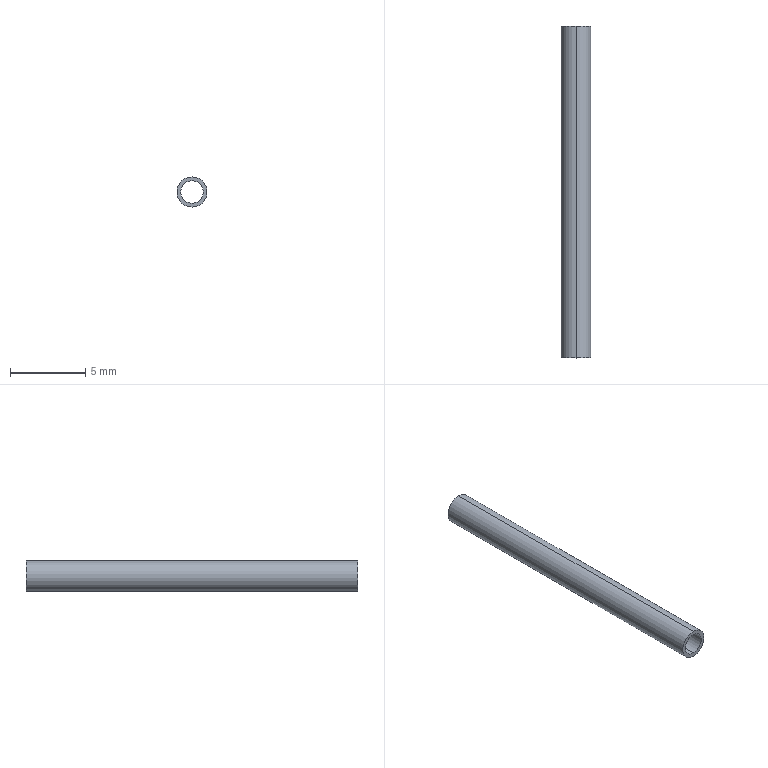Part | SolidWorks | features Revolution 1 | 1 solid | 6 faces | box 2 x 22 x 2 mm | volume 30.238 mm3 | cylinder 4 | plane 2 | commonest cylinder face diameters 1.5 x2 2 x2
STEP:
#1=CARTESIAN_POINT('',(0.,10.2,-1.));
#2=VERTEX_POINT('',#1);
#3=CARTESIAN_POINT('',(0.,10.2,1.));
#4=VERTEX_POINT('',#3);
#5=CARTESIAN_POINT('',(0.,10.2,0.));
#6=DIRECTION('',(0.,-1.,0.));
#7=DIRECTION('',(0.,0.,-1.));
#8=AXIS2_PLACEMENT_3D('',#5,#6,#7);
#9=CIRCLE('',#8,1.);
#10=EDGE_CURVE('',#2,#4,#9,.T.);
#11=ORIENTED_EDGE('',*,*,#10,.T.);
#12=CARTESIAN_POINT('',(0.,-11.8,1.));
#13=VERTEX_POINT('',#12);
#14=CARTESIAN_POINT('',(0.,-14.434,1.));
#15=DIRECTION('',(0.,-1.,0.));
#16=VECTOR('',#15,1000.);
#17=LINE('',#14,#16);
#18=EDGE_CURVE('',#4,#13,#17,.T.);
#19=ORIENTED_EDGE('',*,*,#18,.T.);
#20=CARTESIAN_POINT('',(0.,-11.8,-1.));
#21=VERTEX_POINT('',#20);
#22=CARTESIAN_POINT('',(0.,-11.8,0.));
#23=DIRECTION('',(0.,-1.,0.));
#24=DIRECTION('',(0.,0.,-1.));
#25=AXIS2_PLACEMENT_3D('',#22,#23,#24);
#26=CIRCLE('',#25,1.);
#27=EDGE_CURVE('',#21,#13,#26,.T.);
#28=ORIENTED_EDGE('',*,*,#27,.F.);
#29=CARTESIAN_POINT('',(0.,-14.434,-1.));
#30=DIRECTION('',(0.,-1.,0.));
#31=VECTOR('',#30,1000.);
#32=LINE('',#29,#31);
#33=EDGE_CURVE('',#2,#21,#32,.T.);
#34=ORIENTED_EDGE('',*,*,#33,.F.);
#35=EDGE_LOOP('',(#11,#19,#28,#34));
#36=FACE_OUTER_BOUND('',#35,.T.);
#37=CARTESIAN_POINT('',(0.,-14.434,0.));
#38=DIRECTION('',(0.,-1.,0.));
#39=DIRECTION('',(0.,0.,-1.));
#40=AXIS2_PLACEMENT_3D('',#37,#38,#39);
#41=CYLINDRICAL_SURFACE('',#40,1.);
#42=ADVANCED_FACE('',(#36),#41,.T.);
#43=CARTESIAN_POINT('',(0.,10.2,0.75));
#44=VERTEX_POINT('',#43);
#45=CARTESIAN_POINT('',(0.,10.2,-0.75));
#46=VERTEX_POINT('',#45);
#47=CARTESIAN_POINT('',(0.,10.2,0.));
#48=DIRECTION('',(0.,-1.,0.));
#49=DIRECTION('',(0.,0.,-1.));
#50=AXIS2_PLACEMENT_3D('',#47,#48,#49);
#51=CIRCLE('',#50,0.75);
#52=EDGE_CURVE('',#44,#46,#51,.T.);
#53=ORIENTED_EDGE('',*,*,#52,.F.);
#54=CARTESIAN_POINT('',(0.,-11.8,0.75));
#55=VERTEX_POINT('',#54);
#56=CARTESIAN_POINT('',(0.,-14.434,0.75));
#57=DIRECTION('',(0.,-1.,0.));
#58=VECTOR('',#57,1000.);
#59=LINE('',#56,#58);
#60=EDGE_CURVE('',#44,#55,#59,.T.);
#61=ORIENTED_EDGE('',*,*,#60,.T.);
#62=CARTESIAN_POINT('',(0.,-11.8,-0.75));
#63=VERTEX_POINT('',#62);
#64=CARTESIAN_POINT('',(0.,-11.8,0.));
#65=DIRECTION('',(0.,-1.,0.));
#66=DIRECTION('',(0.,0.,-1.));
#67=AXIS2_PLACEMENT_3D('',#64,#65,#66);
#68=CIRCLE('',#67,0.75);
#69=EDGE_CURVE('',#55,#63,#68,.T.);
#70=ORIENTED_EDGE('',*,*,#69,.T.);
#71=CARTESIAN_POINT('',(0.,-14.434,-0.75));
#72=DIRECTION('',(0.,-1.,0.));
#73=VECTOR('',#72,1000.);
#74=LINE('',#71,#73);
#75=EDGE_CURVE('',#46,#63,#74,.T.);
#76=ORIENTED_EDGE('',*,*,#75,.F.);
#77=EDGE_LOOP('',(#53,#61,#70,#76));
#78=FACE_OUTER_BOUND('',#77,.T.);
#79=CARTESIAN_POINT('',(0.,-14.434,0.));
#80=DIRECTION('',(0.,-1.,0.));
#81=DIRECTION('',(0.,0.,-1.));
#82=AXIS2_PLACEMENT_3D('',#79,#80,#81);
#83=CYLINDRICAL_SURFACE('',#82,0.75);
#84=ADVANCED_FACE('',(#78),#83,.F.);
#85=ORIENTED_EDGE('',*,*,#10,.F.);
#86=CARTESIAN_POINT('',(0.,10.2,0.));
#87=DIRECTION('',(0.,-1.,0.));
#88=DIRECTION('',(0.,0.,-1.));
#89=AXIS2_PLACEMENT_3D('',#86,#87,#88);
#90=CIRCLE('',#89,1.);
#91=EDGE_CURVE('',#4,#2,#90,.T.);
#92=ORIENTED_EDGE('',*,*,#91,.F.);
#93=EDGE_LOOP('',(#85,#92));
#94=FACE_OUTER_BOUND('',#93,.T.);
#95=CARTESIAN_POINT('',(0.,10.2,0.));
#96=DIRECTION('',(0.,-1.,0.));
#97=DIRECTION('',(0.,0.,-1.));
#98=AXIS2_PLACEMENT_3D('',#95,#96,#97);
#99=CIRCLE('',#98,0.75);
#100=EDGE_CURVE('',#46,#44,#99,.T.);
#101=ORIENTED_EDGE('',*,*,#100,.T.);
#102=ORIENTED_EDGE('',*,*,#52,.T.);
#103=EDGE_LOOP('',(#101,#102));
#104=FACE_BOUND('',#103,.T.);
#105=CARTESIAN_POINT('',(-1.,10.2,0.));
#106=DIRECTION('',(0.,-1.,0.));
#107=DIRECTION('',(0.,0.,-1.));
#108=AXIS2_PLACEMENT_3D('',#105,#106,#107);
#109=PLANE('',#108);
#110=ADVANCED_FACE('',(#94,#104),#109,.F.);
#111=ORIENTED_EDGE('',*,*,#60,.F.);
#112=ORIENTED_EDGE('',*,*,#100,.F.);
#113=ORIENTED_EDGE('',*,*,#75,.T.);
#114=CARTESIAN_POINT('',(0.,-11.8,0.));
#115=DIRECTION('',(0.,-1.,0.));
#116=DIRECTION('',(0.,0.,-1.));
#117=AXIS2_PLACEMENT_3D('',#114,#115,#116);
#118=CIRCLE('',#117,0.75);
#119=EDGE_CURVE('',#63,#55,#118,.T.);
#120=ORIENTED_EDGE('',*,*,#119,.T.);
#121=EDGE_LOOP('',(#111,#112,#113,#120));
#122=FACE_OUTER_BOUND('',#121,.T.);
#123=CARTESIAN_POINT('',(0.,-14.434,0.));
#124=DIRECTION('',(0.,-1.,0.));
#125=DIRECTION('',(0.,0.,-1.));
#126=AXIS2_PLACEMENT_3D('',#123,#124,#125);
#127=CYLINDRICAL_SURFACE('',#126,0.75);
#128=ADVANCED_FACE('',(#122),#127,.F.);
#129=ORIENTED_EDGE('',*,*,#119,.F.);
#130=ORIENTED_EDGE('',*,*,#69,.F.);
#131=EDGE_LOOP('',(#129,#130));
#132=FACE_BOUND('',#131,.T.);
#133=ORIENTED_EDGE('',*,*,#27,.T.);
#134=CARTESIAN_POINT('',(0.,-11.8,0.));
#135=DIRECTION('',(0.,-1.,0.));
#136=DIRECTION('',(0.,0.,-1.));
#137=AXIS2_PLACEMENT_3D('',#134,#135,#136);
#138=CIRCLE('',#137,1.);
#139=EDGE_CURVE('',#13,#21,#138,.T.);
#140=ORIENTED_EDGE('',*,*,#139,.T.);
#141=EDGE_LOOP('',(#133,#140));
#142=FACE_OUTER_BOUND('',#141,.T.);
#143=CARTESIAN_POINT('',(-1.,-11.8,0.));
#144=DIRECTION('',(0.,1.,0.));
#145=DIRECTION('',(0.,0.,1.));
#146=AXIS2_PLACEMENT_3D('',#143,#144,#145);
#147=PLANE('',#146);
#148=ADVANCED_FACE('',(#132,#142),#147,.F.);
#149=ORIENTED_EDGE('',*,*,#18,.F.);
#150=ORIENTED_EDGE('',*,*,#91,.T.);
#151=ORIENTED_EDGE('',*,*,#33,.T.);
#152=ORIENTED_EDGE('',*,*,#139,.F.);
#153=EDGE_LOOP('',(#149,#150,#151,#152));
#154=FACE_OUTER_BOUND('',#153,.T.);
#155=CARTESIAN_POINT('',(0.,-14.434,0.));
#156=DIRECTION('',(0.,-1.,0.));
#157=DIRECTION('',(0.,0.,-1.));
#158=AXIS2_PLACEMENT_3D('',#155,#156,#157);
#159=CYLINDRICAL_SURFACE('',#158,1.);
#160=ADVANCED_FACE('',(#154),#159,.T.);
#161=CLOSED_SHELL('',(#42,#84,#110,#128,#148,#160));
#162=MANIFOLD_SOLID_BREP('',#161);
#163=CARTESIAN_POINT('',(0.,0.,0.));
#164=DIRECTION('',(0.,0.,1.));
#165=DIRECTION('',(1.,0.,0.));
#166=AXIS2_PLACEMENT_3D('',#163,#164,#165);
#167=(LENGTH_UNIT()NAMED_UNIT(*)SI_UNIT(.MILLI.,.METRE.));
#168=UNCERTAINTY_MEASURE_WITH_UNIT(LENGTH_MEASURE(0.00001),#167,'','');
#169=(NAMED_UNIT(*)PLANE_ANGLE_UNIT()SI_UNIT($,.RADIAN.));
#170=(NAMED_UNIT(*)SI_UNIT($,.STERADIAN.)SOLID_ANGLE_UNIT());
#171=(GEOMETRIC_REPRESENTATION_CONTEXT(3)GLOBAL_UNCERTAINTY_ASSIGNED_CONTEXT((#168))GLOBAL_UNIT_ASSIGNED_CONTEXT((#167,#169,#170))REPRESENTATION_CONTEXT('',''));
#172=ADVANCED_BREP_SHAPE_REPRESENTATION('',(#162,#166),#171);